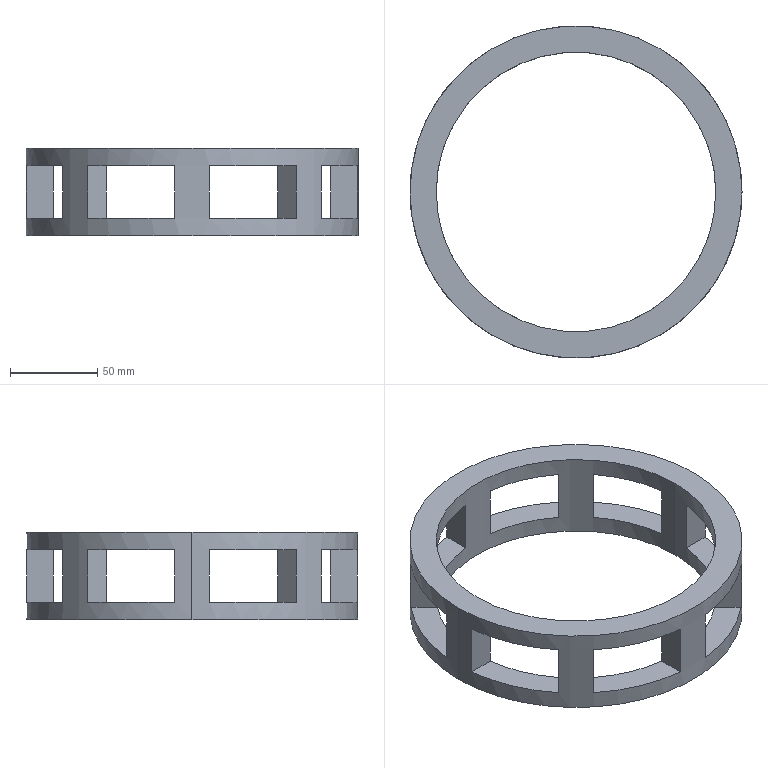Part | SolidWorks | features Cut 1, Extrusion 1 | 1 solid | 38 faces | box 190 x 190 x 50 mm | volume 237092 mm3 | plane 34 | cylinder 4 | commonest cylinder face diameters 160 x2 190 x2
STEP:
#1=CARTESIAN_POINT('',(-536.688,-139.054,40.));
#2=VERTEX_POINT('',#1);
#3=CARTESIAN_POINT('',(-520.512,-100.,40.));
#4=VERTEX_POINT('',#3);
#5=CARTESIAN_POINT('',(-599.884,-90.,40.));
#6=DIRECTION('',(0.,0.,1.));
#7=DIRECTION('',(1.,0.,0.));
#8=AXIS2_PLACEMENT_3D('',#5,#6,#7);
#9=CIRCLE('',#8,80.);
#10=EDGE_CURVE('',#2,#4,#9,.T.);
#11=ORIENTED_EDGE('',*,*,#10,.F.);
#12=CARTESIAN_POINT('',(-536.688,-139.054,10.));
#13=VERTEX_POINT('',#12);
#14=CARTESIAN_POINT('',(-536.688,-139.054,10.));
#15=DIRECTION('',(0.,0.,1.));
#16=VECTOR('',#15,1000.);
#17=LINE('',#14,#16);
#18=EDGE_CURVE('',#13,#2,#17,.T.);
#19=ORIENTED_EDGE('',*,*,#18,.F.);
#20=CARTESIAN_POINT('',(-520.512,-100.,10.));
#21=VERTEX_POINT('',#20);
#22=CARTESIAN_POINT('',(-599.884,-90.,10.));
#23=DIRECTION('',(0.,0.,1.));
#24=DIRECTION('',(1.,0.,0.));
#25=AXIS2_PLACEMENT_3D('',#22,#23,#24);
#26=CIRCLE('',#25,80.);
#27=EDGE_CURVE('',#13,#21,#26,.T.);
#28=ORIENTED_EDGE('',*,*,#27,.T.);
#29=CARTESIAN_POINT('',(-520.512,-100.,10.));
#30=DIRECTION('',(0.,0.,-1.));
#31=VECTOR('',#30,1000.);
#32=LINE('',#29,#31);
#33=EDGE_CURVE('',#4,#21,#32,.T.);
#34=ORIENTED_EDGE('',*,*,#33,.F.);
#35=EDGE_LOOP('',(#11,#19,#28,#34));
#36=FACE_BOUND('',#35,.T.);
#37=CARTESIAN_POINT('',(-589.884,-169.373,40.));
#38=VERTEX_POINT('',#37);
#39=CARTESIAN_POINT('',(-550.83,-153.196,40.));
#40=VERTEX_POINT('',#39);
#41=CARTESIAN_POINT('',(-599.884,-90.,40.));
#42=DIRECTION('',(0.,0.,1.));
#43=DIRECTION('',(1.,0.,0.));
#44=AXIS2_PLACEMENT_3D('',#41,#42,#43);
#45=CIRCLE('',#44,80.);
#46=EDGE_CURVE('',#38,#40,#45,.T.);
#47=ORIENTED_EDGE('',*,*,#46,.F.);
#48=CARTESIAN_POINT('',(-589.884,-169.373,10.));
#49=VERTEX_POINT('',#48);
#50=CARTESIAN_POINT('',(-589.884,-169.373,10.));
#51=DIRECTION('',(0.,0.,-1.));
#52=VECTOR('',#51,1000.);
#53=LINE('',#50,#52);
#54=EDGE_CURVE('',#38,#49,#53,.T.);
#55=ORIENTED_EDGE('',*,*,#54,.T.);
#56=CARTESIAN_POINT('',(-550.83,-153.196,10.));
#57=VERTEX_POINT('',#56);
#58=CARTESIAN_POINT('',(-599.884,-90.,10.));
#59=DIRECTION('',(0.,0.,1.));
#60=DIRECTION('',(1.,0.,0.));
#61=AXIS2_PLACEMENT_3D('',#58,#59,#60);
#62=CIRCLE('',#61,80.);
#63=EDGE_CURVE('',#49,#57,#62,.T.);
#64=ORIENTED_EDGE('',*,*,#63,.T.);
#65=CARTESIAN_POINT('',(-550.83,-153.196,10.));
#66=DIRECTION('',(0.,0.,1.));
#67=VECTOR('',#66,1000.);
#68=LINE('',#65,#67);
#69=EDGE_CURVE('',#57,#40,#68,.T.);
#70=ORIENTED_EDGE('',*,*,#69,.T.);
#71=EDGE_LOOP('',(#47,#55,#64,#70));
#72=FACE_BOUND('',#71,.T.);
#73=CARTESIAN_POINT('',(-648.938,-153.196,40.));
#74=VERTEX_POINT('',#73);
#75=CARTESIAN_POINT('',(-609.884,-169.373,40.));
#76=VERTEX_POINT('',#75);
#77=CARTESIAN_POINT('',(-599.884,-90.,40.));
#78=DIRECTION('',(0.,0.,1.));
#79=DIRECTION('',(1.,0.,0.));
#80=AXIS2_PLACEMENT_3D('',#77,#78,#79);
#81=CIRCLE('',#80,80.);
#82=EDGE_CURVE('',#74,#76,#81,.T.);
#83=ORIENTED_EDGE('',*,*,#82,.F.);
#84=CARTESIAN_POINT('',(-648.938,-153.196,10.));
#85=VERTEX_POINT('',#84);
#86=CARTESIAN_POINT('',(-648.938,-153.196,10.));
#87=DIRECTION('',(0.,0.,-1.));
#88=VECTOR('',#87,1000.);
#89=LINE('',#86,#88);
#90=EDGE_CURVE('',#74,#85,#89,.T.);
#91=ORIENTED_EDGE('',*,*,#90,.T.);
#92=CARTESIAN_POINT('',(-609.884,-169.373,10.));
#93=VERTEX_POINT('',#92);
#94=CARTESIAN_POINT('',(-599.884,-90.,10.));
#95=DIRECTION('',(0.,0.,1.));
#96=DIRECTION('',(1.,0.,0.));
#97=AXIS2_PLACEMENT_3D('',#94,#95,#96);
#98=CIRCLE('',#97,80.);
#99=EDGE_CURVE('',#85,#93,#98,.T.);
#100=ORIENTED_EDGE('',*,*,#99,.T.);
#101=CARTESIAN_POINT('',(-609.884,-169.373,10.));
#102=DIRECTION('',(0.,0.,-1.));
#103=VECTOR('',#102,1000.);
#104=LINE('',#101,#103);
#105=EDGE_CURVE('',#76,#93,#104,.T.);
#106=ORIENTED_EDGE('',*,*,#105,.F.);
#107=EDGE_LOOP('',(#83,#91,#100,#106));
#108=FACE_BOUND('',#107,.T.);
#109=CARTESIAN_POINT('',(-679.257,-100.,40.));
#110=VERTEX_POINT('',#109);
#111=CARTESIAN_POINT('',(-663.08,-139.054,40.));
#112=VERTEX_POINT('',#111);
#113=CARTESIAN_POINT('',(-599.884,-90.,40.));
#114=DIRECTION('',(0.,0.,1.));
#115=DIRECTION('',(1.,0.,0.));
#116=AXIS2_PLACEMENT_3D('',#113,#114,#115);
#117=CIRCLE('',#116,80.);
#118=EDGE_CURVE('',#110,#112,#117,.T.);
#119=ORIENTED_EDGE('',*,*,#118,.F.);
#120=CARTESIAN_POINT('',(-679.257,-100.,10.));
#121=VERTEX_POINT('',#120);
#122=CARTESIAN_POINT('',(-679.257,-100.,10.));
#123=DIRECTION('',(0.,0.,1.));
#124=VECTOR('',#123,1000.);
#125=LINE('',#122,#124);
#126=EDGE_CURVE('',#121,#110,#125,.T.);
#127=ORIENTED_EDGE('',*,*,#126,.F.);
#128=CARTESIAN_POINT('',(-663.08,-139.054,10.));
#129=VERTEX_POINT('',#128);
#130=CARTESIAN_POINT('',(-599.884,-90.,10.));
#131=DIRECTION('',(0.,0.,1.));
#132=DIRECTION('',(1.,0.,0.));
#133=AXIS2_PLACEMENT_3D('',#130,#131,#132);
#134=CIRCLE('',#133,80.);
#135=EDGE_CURVE('',#121,#129,#134,.T.);
#136=ORIENTED_EDGE('',*,*,#135,.T.);
#137=CARTESIAN_POINT('',(-663.08,-139.054,10.));
#138=DIRECTION('',(0.,0.,-1.));
#139=VECTOR('',#138,1000.);
#140=LINE('',#137,#139);
#141=EDGE_CURVE('',#112,#129,#140,.T.);
#142=ORIENTED_EDGE('',*,*,#141,.F.);
#143=EDGE_LOOP('',(#119,#127,#136,#142));
#144=FACE_BOUND('',#143,.T.);
#145=CARTESIAN_POINT('',(-679.884,-90.,50.));
#146=VERTEX_POINT('',#145);
#147=CARTESIAN_POINT('',(-519.884,-90.,50.));
#148=VERTEX_POINT('',#147);
#149=CARTESIAN_POINT('',(-599.884,-90.,50.));
#150=DIRECTION('',(0.,0.,1.));
#151=DIRECTION('',(1.,0.,0.));
#152=AXIS2_PLACEMENT_3D('',#149,#150,#151);
#153=CIRCLE('',#152,80.);
#154=EDGE_CURVE('',#146,#148,#153,.T.);
#155=ORIENTED_EDGE('',*,*,#154,.T.);
#156=CARTESIAN_POINT('',(-519.884,-90.,0.));
#157=VERTEX_POINT('',#156);
#158=CARTESIAN_POINT('',(-519.884,-90.,50.));
#159=DIRECTION('',(0.,0.,-1.));
#160=VECTOR('',#159,1000.);
#161=LINE('',#158,#160);
#162=EDGE_CURVE('',#148,#157,#161,.T.);
#163=ORIENTED_EDGE('',*,*,#162,.T.);
#164=CARTESIAN_POINT('',(-679.884,-90.,0.));
#165=VERTEX_POINT('',#164);
#166=CARTESIAN_POINT('',(-599.884,-90.,0.));
#167=DIRECTION('',(0.,0.,1.));
#168=DIRECTION('',(1.,0.,0.));
#169=AXIS2_PLACEMENT_3D('',#166,#167,#168);
#170=CIRCLE('',#169,80.);
#171=EDGE_CURVE('',#165,#157,#170,.T.);
#172=ORIENTED_EDGE('',*,*,#171,.F.);
#173=CARTESIAN_POINT('',(-679.884,-90.,50.));
#174=DIRECTION('',(0.,0.,-1.));
#175=VECTOR('',#174,1000.);
#176=LINE('',#173,#175);
#177=EDGE_CURVE('',#146,#165,#176,.T.);
#178=ORIENTED_EDGE('',*,*,#177,.F.);
#179=EDGE_LOOP('',(#155,#163,#172,#178));
#180=FACE_OUTER_BOUND('',#179,.T.);
#181=CARTESIAN_POINT('',(-599.884,-90.,50.));
#182=DIRECTION('',(0.,0.,-1.));
#183=DIRECTION('',(-1.,0.,0.));
#184=AXIS2_PLACEMENT_3D('',#181,#182,#183);
#185=CYLINDRICAL_SURFACE('',#184,80.);
#186=ADVANCED_FACE('',(#36,#72,#108,#144,#180),#185,.F.);
#187=CARTESIAN_POINT('',(-589.884,4.472,10.));
#188=VERTEX_POINT('',#187);
#189=CARTESIAN_POINT('',(-589.884,4.472,40.));
#190=VERTEX_POINT('',#189);
#191=CARTESIAN_POINT('',(-589.884,4.472,10.));
#192=DIRECTION('',(0.,0.,1.));
#193=VECTOR('',#192,1000.);
#194=LINE('',#191,#193);
#195=EDGE_CURVE('',#188,#190,#194,.T.);
#196=ORIENTED_EDGE('',*,*,#195,.F.);
#197=CARTESIAN_POINT('',(-540.153,-16.127,10.));
#198=VERTEX_POINT('',#197);
#199=CARTESIAN_POINT('',(-599.884,-90.,10.));
#200=DIRECTION('',(0.,0.,1.));
#201=DIRECTION('',(1.,0.,0.));
#202=AXIS2_PLACEMENT_3D('',#199,#200,#201);
#203=CIRCLE('',#202,95.);
#204=EDGE_CURVE('',#198,#188,#203,.T.);
#205=ORIENTED_EDGE('',*,*,#204,.F.);
#206=CARTESIAN_POINT('',(-540.153,-16.127,40.));
#207=VERTEX_POINT('',#206);
#208=CARTESIAN_POINT('',(-540.153,-16.127,10.));
#209=DIRECTION('',(0.,0.,1.));
#210=VECTOR('',#209,1000.);
#211=LINE('',#208,#210);
#212=EDGE_CURVE('',#198,#207,#211,.T.);
#213=ORIENTED_EDGE('',*,*,#212,.T.);
#214=CARTESIAN_POINT('',(-599.884,-90.,40.));
#215=DIRECTION('',(0.,0.,1.));
#216=DIRECTION('',(1.,0.,0.));
#217=AXIS2_PLACEMENT_3D('',#214,#215,#216);
#218=CIRCLE('',#217,95.);
#219=EDGE_CURVE('',#207,#190,#218,.T.);
#220=ORIENTED_EDGE('',*,*,#219,.T.);
#221=EDGE_LOOP('',(#196,#205,#213,#220));
#222=FACE_BOUND('',#221,.T.);
#223=CARTESIAN_POINT('',(-673.757,-30.269,10.));
#224=VERTEX_POINT('',#223);
#225=CARTESIAN_POINT('',(-673.757,-30.269,40.));
#226=VERTEX_POINT('',#225);
#227=CARTESIAN_POINT('',(-673.757,-30.269,10.));
#228=DIRECTION('',(0.,0.,1.));
#229=VECTOR('',#228,1000.);
#230=LINE('',#227,#229);
#231=EDGE_CURVE('',#224,#226,#230,.T.);
#232=ORIENTED_EDGE('',*,*,#231,.T.);
#233=CARTESIAN_POINT('',(-694.356,-80.,40.));
#234=VERTEX_POINT('',#233);
#235=CARTESIAN_POINT('',(-599.884,-90.,40.));
#236=DIRECTION('',(0.,0.,1.));
#237=DIRECTION('',(1.,0.,0.));
#238=AXIS2_PLACEMENT_3D('',#235,#236,#237);
#239=CIRCLE('',#238,95.);
#240=EDGE_CURVE('',#226,#234,#239,.T.);
#241=ORIENTED_EDGE('',*,*,#240,.T.);
#242=CARTESIAN_POINT('',(-694.356,-80.,10.));
#243=VERTEX_POINT('',#242);
#244=CARTESIAN_POINT('',(-694.356,-80.,10.));
#245=DIRECTION('',(0.,0.,1.));
#246=VECTOR('',#245,1000.);
#247=LINE('',#244,#246);
#248=EDGE_CURVE('',#243,#234,#247,.T.);
#249=ORIENTED_EDGE('',*,*,#248,.F.);
#250=CARTESIAN_POINT('',(-599.884,-90.,10.));
#251=DIRECTION('',(0.,0.,1.));
#252=DIRECTION('',(1.,0.,0.));
#253=AXIS2_PLACEMENT_3D('',#250,#251,#252);
#254=CIRCLE('',#253,95.);
#255=EDGE_CURVE('',#224,#243,#254,.T.);
#256=ORIENTED_EDGE('',*,*,#255,.F.);
#257=EDGE_LOOP('',(#232,#241,#249,#256));
#258=FACE_BOUND('',#257,.T.);
#259=CARTESIAN_POINT('',(-526.011,-30.269,10.));
#260=VERTEX_POINT('',#259);
#261=CARTESIAN_POINT('',(-526.011,-30.269,40.));
#262=VERTEX_POINT('',#261);
#263=CARTESIAN_POINT('',(-526.011,-30.269,10.));
#264=DIRECTION('',(0.,0.,1.));
#265=VECTOR('',#264,1000.);
#266=LINE('',#263,#265);
#267=EDGE_CURVE('',#260,#262,#266,.T.);
#268=ORIENTED_EDGE('',*,*,#267,.F.);
#269=CARTESIAN_POINT('',(-505.412,-80.,10.));
#270=VERTEX_POINT('',#269);
#271=CARTESIAN_POINT('',(-599.884,-90.,10.));
#272=DIRECTION('',(0.,0.,1.));
#273=DIRECTION('',(1.,0.,0.));
#274=AXIS2_PLACEMENT_3D('',#271,#272,#273);
#275=CIRCLE('',#274,95.);
#276=EDGE_CURVE('',#270,#260,#275,.T.);
#277=ORIENTED_EDGE('',*,*,#276,.F.);
#278=CARTESIAN_POINT('',(-505.412,-80.,40.));
#279=VERTEX_POINT('',#278);
#280=CARTESIAN_POINT('',(-505.412,-80.,10.));
#281=DIRECTION('',(0.,0.,1.));
#282=VECTOR('',#281,1000.);
#283=LINE('',#280,#282);
#284=EDGE_CURVE('',#270,#279,#283,.T.);
#285=ORIENTED_EDGE('',*,*,#284,.T.);
#286=CARTESIAN_POINT('',(-599.884,-90.,40.));
#287=DIRECTION('',(0.,0.,1.));
#288=DIRECTION('',(1.,0.,0.));
#289=AXIS2_PLACEMENT_3D('',#286,#287,#288);
#290=CIRCLE('',#289,95.);
#291=EDGE_CURVE('',#279,#262,#290,.T.);
#292=ORIENTED_EDGE('',*,*,#291,.T.);
#293=EDGE_LOOP('',(#268,#277,#285,#292));
#294=FACE_BOUND('',#293,.T.);
#295=CARTESIAN_POINT('',(-609.884,4.472,40.));
#296=VERTEX_POINT('',#295);
#297=CARTESIAN_POINT('',(-659.615,-16.127,40.));
#298=VERTEX_POINT('',#297);
#299=CARTESIAN_POINT('',(-599.884,-90.,40.));
#300=DIRECTION('',(0.,0.,1.));
#301=DIRECTION('',(1.,0.,0.));
#302=AXIS2_PLACEMENT_3D('',#299,#300,#301);
#303=CIRCLE('',#302,95.);
#304=EDGE_CURVE('',#296,#298,#303,.T.);
#305=ORIENTED_EDGE('',*,*,#304,.T.);
#306=CARTESIAN_POINT('',(-659.615,-16.127,10.));
#307=VERTEX_POINT('',#306);
#308=CARTESIAN_POINT('',(-659.615,-16.127,10.));
#309=DIRECTION('',(0.,0.,1.));
#310=VECTOR('',#309,1000.);
#311=LINE('',#308,#310);
#312=EDGE_CURVE('',#307,#298,#311,.T.);
#313=ORIENTED_EDGE('',*,*,#312,.F.);
#314=CARTESIAN_POINT('',(-609.884,4.472,10.));
#315=VERTEX_POINT('',#314);
#316=CARTESIAN_POINT('',(-599.884,-90.,10.));
#317=DIRECTION('',(0.,0.,1.));
#318=DIRECTION('',(1.,0.,0.));
#319=AXIS2_PLACEMENT_3D('',#316,#317,#318);
#320=CIRCLE('',#319,95.);
#321=EDGE_CURVE('',#315,#307,#320,.T.);
#322=ORIENTED_EDGE('',*,*,#321,.F.);
#323=CARTESIAN_POINT('',(-609.884,4.472,10.));
#324=DIRECTION('',(0.,0.,1.));
#325=VECTOR('',#324,1000.);
#326=LINE('',#323,#325);
#327=EDGE_CURVE('',#315,#296,#326,.T.);
#328=ORIENTED_EDGE('',*,*,#327,.T.);
#329=EDGE_LOOP('',(#305,#313,#322,#328));
#330=FACE_BOUND('',#329,.T.);
#331=CARTESIAN_POINT('',(-504.884,-90.,50.));
#332=VERTEX_POINT('',#331);
#333=CARTESIAN_POINT('',(-694.884,-90.,50.));
#334=VERTEX_POINT('',#333);
#335=CARTESIAN_POINT('',(-599.884,-90.,50.));
#336=DIRECTION('',(0.,0.,1.));
#337=DIRECTION('',(1.,0.,0.));
#338=AXIS2_PLACEMENT_3D('',#335,#336,#337);
#339=CIRCLE('',#338,95.);
#340=EDGE_CURVE('',#332,#334,#339,.T.);
#341=ORIENTED_EDGE('',*,*,#340,.F.);
#342=CARTESIAN_POINT('',(-504.884,-90.,0.));
#343=VERTEX_POINT('',#342);
#344=CARTESIAN_POINT('',(-504.884,-90.,50.));
#345=DIRECTION('',(0.,0.,-1.));
#346=VECTOR('',#345,1000.);
#347=LINE('',#344,#346);
#348=EDGE_CURVE('',#332,#343,#347,.T.);
#349=ORIENTED_EDGE('',*,*,#348,.T.);
#350=CARTESIAN_POINT('',(-694.884,-90.,0.));
#351=VERTEX_POINT('',#350);
#352=CARTESIAN_POINT('',(-599.884,-90.,0.));
#353=DIRECTION('',(0.,0.,1.));
#354=DIRECTION('',(1.,0.,0.));
#355=AXIS2_PLACEMENT_3D('',#352,#353,#354);
#356=CIRCLE('',#355,95.);
#357=EDGE_CURVE('',#343,#351,#356,.T.);
#358=ORIENTED_EDGE('',*,*,#357,.T.);
#359=CARTESIAN_POINT('',(-694.884,-90.,50.));
#360=DIRECTION('',(0.,0.,-1.));
#361=VECTOR('',#360,1000.);
#362=LINE('',#359,#361);
#363=EDGE_CURVE('',#334,#351,#362,.T.);
#364=ORIENTED_EDGE('',*,*,#363,.F.);
#365=EDGE_LOOP('',(#341,#349,#358,#364));
#366=FACE_OUTER_BOUND('',#365,.T.);
#367=CARTESIAN_POINT('',(-599.884,-90.,50.));
#368=DIRECTION('',(0.,0.,-1.));
#369=DIRECTION('',(-1.,0.,0.));
#370=AXIS2_PLACEMENT_3D('',#367,#368,#369);
#371=CYLINDRICAL_SURFACE('',#370,95.);
#372=ADVANCED_FACE('',(#222,#258,#294,#330,#366),#371,.T.);
#373=ORIENTED_EDGE('',*,*,#348,.F.);
#374=CARTESIAN_POINT('',(-599.884,-90.,50.));
#375=DIRECTION('',(0.,0.,1.));
#376=DIRECTION('',(1.,0.,0.));
#377=AXIS2_PLACEMENT_3D('',#374,#375,#376);
#378=CIRCLE('',#377,95.);
#379=EDGE_CURVE('',#334,#332,#378,.T.);
#380=ORIENTED_EDGE('',*,*,#379,.F.);
#381=ORIENTED_EDGE('',*,*,#363,.T.);
#382=CARTESIAN_POINT('',(-599.884,-90.,0.));
#383=DIRECTION('',(0.,0.,1.));
#384=DIRECTION('',(1.,0.,0.));
#385=AXIS2_PLACEMENT_3D('',#382,#383,#384);
#386=CIRCLE('',#385,95.);
#387=EDGE_CURVE('',#351,#343,#386,.T.);
#388=ORIENTED_EDGE('',*,*,#387,.T.);
#389=EDGE_LOOP('',(#373,#380,#381,#388));
#390=FACE_OUTER_BOUND('',#389,.T.);
#391=CARTESIAN_POINT('',(-694.356,-100.,10.));
#392=VERTEX_POINT('',#391);
#393=CARTESIAN_POINT('',(-694.356,-100.,40.));
#394=VERTEX_POINT('',#393);
#395=CARTESIAN_POINT('',(-694.356,-100.,10.));
#396=DIRECTION('',(0.,0.,1.));
#397=VECTOR('',#396,1000.);
#398=LINE('',#395,#397);
#399=EDGE_CURVE('',#392,#394,#398,.T.);
#400=ORIENTED_EDGE('',*,*,#399,.T.);
#401=CARTESIAN_POINT('',(-673.757,-149.731,40.));
#402=VERTEX_POINT('',#401);
#403=CARTESIAN_POINT('',(-599.884,-90.,40.));
#404=DIRECTION('',(0.,0.,1.));
#405=DIRECTION('',(1.,0.,0.));
#406=AXIS2_PLACEMENT_3D('',#403,#404,#405);
#407=CIRCLE('',#406,95.);
#408=EDGE_CURVE('',#394,#402,#407,.T.);
#409=ORIENTED_EDGE('',*,*,#408,.T.);
#410=CARTESIAN_POINT('',(-673.757,-149.731,10.));
#411=VERTEX_POINT('',#410);
#412=CARTESIAN_POINT('',(-673.757,-149.731,10.));
#413=DIRECTION('',(0.,0.,1.));
#414=VECTOR('',#413,1000.);
#415=LINE('',#412,#414);
#416=EDGE_CURVE('',#411,#402,#415,.T.);
#417=ORIENTED_EDGE('',*,*,#416,.F.);
#418=CARTESIAN_POINT('',(-599.884,-90.,10.));
#419=DIRECTION('',(0.,0.,1.));
#420=DIRECTION('',(1.,0.,0.));
#421=AXIS2_PLACEMENT_3D('',#418,#419,#420);
#422=CIRCLE('',#421,95.);
#423=EDGE_CURVE('',#392,#411,#422,.T.);
#424=ORIENTED_EDGE('',*,*,#423,.F.);
#425=EDGE_LOOP('',(#400,#409,#417,#424));
#426=FACE_BOUND('',#425,.T.);
#427=CARTESIAN_POINT('',(-526.011,-149.731,40.));
#428=VERTEX_POINT('',#427);
#429=CARTESIAN_POINT('',(-505.412,-100.,40.));
#430=VERTEX_POINT('',#429);
#431=CARTESIAN_POINT('',(-599.884,-90.,40.));
#432=DIRECTION('',(0.,0.,1.));
#433=DIRECTION('',(1.,0.,0.));
#434=AXIS2_PLACEMENT_3D('',#431,#432,#433);
#435=CIRCLE('',#434,95.);
#436=EDGE_CURVE('',#428,#430,#435,.T.);
#437=ORIENTED_EDGE('',*,*,#436,.T.);
#438=CARTESIAN_POINT('',(-505.412,-100.,10.));
#439=VERTEX_POINT('',#438);
#440=CARTESIAN_POINT('',(-505.412,-100.,10.));
#441=DIRECTION('',(0.,0.,1.));
#442=VECTOR('',#441,1000.);
#443=LINE('',#440,#442);
#444=EDGE_CURVE('',#439,#430,#443,.T.);
#445=ORIENTED_EDGE('',*,*,#444,.F.);
#446=CARTESIAN_POINT('',(-526.011,-149.731,10.));
#447=VERTEX_POINT('',#446);
#448=CARTESIAN_POINT('',(-599.884,-90.,10.));
#449=DIRECTION('',(0.,0.,1.));
#450=DIRECTION('',(1.,0.,0.));
#451=AXIS2_PLACEMENT_3D('',#448,#449,#450);
#452=CIRCLE('',#451,95.);
#453=EDGE_CURVE('',#447,#439,#452,.T.);
#454=ORIENTED_EDGE('',*,*,#453,.F.);
#455=CARTESIAN_POINT('',(-526.011,-149.731,10.));
#456=DIRECTION('',(0.,0.,1.));
#457=VECTOR('',#456,1000.);
#458=LINE('',#455,#457);
#459=EDGE_CURVE('',#447,#428,#458,.T.);
#460=ORIENTED_EDGE('',*,*,#459,.T.);
#461=EDGE_LOOP('',(#437,#445,#454,#460));
#462=FACE_BOUND('',#461,.T.);
#463=CARTESIAN_POINT('',(-659.615,-163.873,40.));
#464=VERTEX_POINT('',#463);
#465=CARTESIAN_POINT('',(-609.884,-184.472,40.));
#466=VERTEX_POINT('',#465);
#467=CARTESIAN_POINT('',(-599.884,-90.,40.));
#468=DIRECTION('',(0.,0.,1.));
#469=DIRECTION('',(1.,0.,0.));
#470=AXIS2_PLACEMENT_3D('',#467,#468,#469);
#471=CIRCLE('',#470,95.);
#472=EDGE_CURVE('',#464,#466,#471,.T.);
#473=ORIENTED_EDGE('',*,*,#472,.T.);
#474=CARTESIAN_POINT('',(-609.884,-184.472,10.));
#475=VERTEX_POINT('',#474);
#476=CARTESIAN_POINT('',(-609.884,-184.472,10.));
#477=DIRECTION('',(0.,0.,1.));
#478=VECTOR('',#477,1000.);
#479=LINE('',#476,#478);
#480=EDGE_CURVE('',#475,#466,#479,.T.);
#481=ORIENTED_EDGE('',*,*,#480,.F.);
#482=CARTESIAN_POINT('',(-659.615,-163.873,10.));
#483=VERTEX_POINT('',#482);
#484=CARTESIAN_POINT('',(-599.884,-90.,10.));
#485=DIRECTION('',(0.,0.,1.));
#486=DIRECTION('',(1.,0.,0.));
#487=AXIS2_PLACEMENT_3D('',#484,#485,#486);
#488=CIRCLE('',#487,95.);
#489=EDGE_CURVE('',#483,#475,#488,.T.);
#490=ORIENTED_EDGE('',*,*,#489,.F.);
#491=CARTESIAN_POINT('',(-659.615,-163.873,10.));
#492=DIRECTION('',(0.,0.,1.));
#493=VECTOR('',#492,1000.);
#494=LINE('',#491,#493);
#495=EDGE_CURVE('',#483,#464,#494,.T.);
#496=ORIENTED_EDGE('',*,*,#495,.T.);
#497=EDGE_LOOP('',(#473,#481,#490,#496));
#498=FACE_BOUND('',#497,.T.);
#499=CARTESIAN_POINT('',(-540.153,-163.873,10.));
#500=VERTEX_POINT('',#499);
#501=CARTESIAN_POINT('',(-540.153,-163.873,40.));
#502=VERTEX_POINT('',#501);
#503=CARTESIAN_POINT('',(-540.153,-163.873,10.));
#504=DIRECTION('',(0.,0.,1.));
#505=VECTOR('',#504,1000.);
#506=LINE('',#503,#505);
#507=EDGE_CURVE('',#500,#502,#506,.T.);
#508=ORIENTED_EDGE('',*,*,#507,.F.);
#509=CARTESIAN_POINT('',(-589.884,-184.472,10.));
#510=VERTEX_POINT('',#509);
#511=CARTESIAN_POINT('',(-599.884,-90.,10.));
#512=DIRECTION('',(0.,0.,1.));
#513=DIRECTION('',(1.,0.,0.));
#514=AXIS2_PLACEMENT_3D('',#511,#512,#513);
#515=CIRCLE('',#514,95.);
#516=EDGE_CURVE('',#510,#500,#515,.T.);
#517=ORIENTED_EDGE('',*,*,#516,.F.);
#518=CARTESIAN_POINT('',(-589.884,-184.472,40.));
#519=VERTEX_POINT('',#518);
#520=CARTESIAN_POINT('',(-589.884,-184.472,10.));
#521=DIRECTION('',(0.,0.,1.));
#522=VECTOR('',#521,1000.);
#523=LINE('',#520,#522);
#524=EDGE_CURVE('',#510,#519,#523,.T.);
#525=ORIENTED_EDGE('',*,*,#524,.T.);
#526=CARTESIAN_POINT('',(-599.884,-90.,40.));
#527=DIRECTION('',(0.,0.,1.));
#528=DIRECTION('',(1.,0.,0.));
#529=AXIS2_PLACEMENT_3D('',#526,#527,#528);
#530=CIRCLE('',#529,95.);
#531=EDGE_CURVE('',#519,#502,#530,.T.);
#532=ORIENTED_EDGE('',*,*,#531,.T.);
#533=EDGE_LOOP('',(#508,#517,#525,#532));
#534=FACE_BOUND('',#533,.T.);
#535=CARTESIAN_POINT('',(-599.884,-90.,50.));
#536=DIRECTION('',(0.,0.,-1.));
#537=DIRECTION('',(-1.,0.,0.));
#538=AXIS2_PLACEMENT_3D('',#535,#536,#537);
#539=CYLINDRICAL_SURFACE('',#538,95.);
#540=ADVANCED_FACE('',(#390,#426,#462,#498,#534),#539,.T.);
#541=ORIENTED_EDGE('',*,*,#162,.F.);
#542=CARTESIAN_POINT('',(-599.884,-90.,50.));
#543=DIRECTION('',(0.,0.,1.));
#544=DIRECTION('',(1.,0.,0.));
#545=AXIS2_PLACEMENT_3D('',#542,#543,#544);
#546=CIRCLE('',#545,80.);
#547=EDGE_CURVE('',#148,#146,#546,.T.);
#548=ORIENTED_EDGE('',*,*,#547,.T.);
#549=ORIENTED_EDGE('',*,*,#177,.T.);
#550=CARTESIAN_POINT('',(-599.884,-90.,0.));
#551=DIRECTION('',(0.,0.,1.));
#552=DIRECTION('',(1.,0.,0.));
#553=AXIS2_PLACEMENT_3D('',#550,#551,#552);
#554=CIRCLE('',#553,80.);
#555=EDGE_CURVE('',#157,#165,#554,.T.);
#556=ORIENTED_EDGE('',*,*,#555,.F.);
#557=EDGE_LOOP('',(#541,#548,#549,#556));
#558=FACE_OUTER_BOUND('',#557,.T.);
#559=CARTESIAN_POINT('',(-550.83,-26.804,40.));
#560=VERTEX_POINT('',#559);
#561=CARTESIAN_POINT('',(-589.884,-10.627,40.));
#562=VERTEX_POINT('',#561);
#563=CARTESIAN_POINT('',(-599.884,-90.,40.));
#564=DIRECTION('',(0.,0.,1.));
#565=DIRECTION('',(1.,0.,0.));
#566=AXIS2_PLACEMENT_3D('',#563,#564,#565);
#567=CIRCLE('',#566,80.);
#568=EDGE_CURVE('',#560,#562,#567,.T.);
#569=ORIENTED_EDGE('',*,*,#568,.F.);
#570=CARTESIAN_POINT('',(-550.83,-26.804,10.));
#571=VERTEX_POINT('',#570);
#572=CARTESIAN_POINT('',(-550.83,-26.804,10.));
#573=DIRECTION('',(0.,0.,1.));
#574=VECTOR('',#573,1000.);
#575=LINE('',#572,#574);
#576=EDGE_CURVE('',#571,#560,#575,.T.);
#577=ORIENTED_EDGE('',*,*,#576,.F.);
#578=CARTESIAN_POINT('',(-589.884,-10.627,10.));
#579=VERTEX_POINT('',#578);
#580=CARTESIAN_POINT('',(-599.884,-90.,10.));
#581=DIRECTION('',(0.,0.,1.));
#582=DIRECTION('',(1.,0.,0.));
#583=AXIS2_PLACEMENT_3D('',#580,#581,#582);
#584=CIRCLE('',#583,80.);
#585=EDGE_CURVE('',#571,#579,#584,.T.);
#586=ORIENTED_EDGE('',*,*,#585,.T.);
#587=CARTESIAN_POINT('',(-589.884,-10.627,10.));
#588=DIRECTION('',(0.,0.,1.));
#589=VECTOR('',#588,1000.);
#590=LINE('',#587,#589);
#591=EDGE_CURVE('',#579,#562,#590,.T.);
#592=ORIENTED_EDGE('',*,*,#591,.T.);
#593=EDGE_LOOP('',(#569,#577,#586,#592));
#594=FACE_BOUND('',#593,.T.);
#595=CARTESIAN_POINT('',(-609.884,-10.627,40.));
#596=VERTEX_POINT('',#595);
#597=CARTESIAN_POINT('',(-648.938,-26.804,40.));
#598=VERTEX_POINT('',#597);
#599=CARTESIAN_POINT('',(-599.884,-90.,40.));
#600=DIRECTION('',(0.,0.,1.));
#601=DIRECTION('',(1.,0.,0.));
#602=AXIS2_PLACEMENT_3D('',#599,#600,#601);
#603=CIRCLE('',#602,80.);
#604=EDGE_CURVE('',#596,#598,#603,.T.);
#605=ORIENTED_EDGE('',*,*,#604,.F.);
#606=CARTESIAN_POINT('',(-609.884,-10.627,10.));
#607=VERTEX_POINT('',#606);
#608=CARTESIAN_POINT('',(-609.884,-10.627,10.));
#609=DIRECTION('',(0.,0.,1.));
#610=VECTOR('',#609,1000.);
#611=LINE('',#608,#610);
#612=EDGE_CURVE('',#607,#596,#611,.T.);
#613=ORIENTED_EDGE('',*,*,#612,.F.);
#614=CARTESIAN_POINT('',(-648.938,-26.804,10.));
#615=VERTEX_POINT('',#614);
#616=CARTESIAN_POINT('',(-599.884,-90.,10.));
#617=DIRECTION('',(0.,0.,1.));
#618=DIRECTION('',(1.,0.,0.));
#619=AXIS2_PLACEMENT_3D('',#616,#617,#618);
#620=CIRCLE('',#619,80.);
#621=EDGE_CURVE('',#607,#615,#620,.T.);
#622=ORIENTED_EDGE('',*,*,#621,.T.);
#623=CARTESIAN_POINT('',(-648.938,-26.804,10.));
#624=DIRECTION('',(0.,0.,-1.));
#625=VECTOR('',#624,1000.);
#626=LINE('',#623,#625);
#627=EDGE_CURVE('',#598,#615,#626,.T.);
#628=ORIENTED_EDGE('',*,*,#627,.F.);
#629=EDGE_LOOP('',(#605,#613,#622,#628));
#630=FACE_BOUND('',#629,.T.);
#631=CARTESIAN_POINT('',(-663.08,-40.946,40.));
#632=VERTEX_POINT('',#631);
#633=CARTESIAN_POINT('',(-679.257,-80.,40.));
#634=VERTEX_POINT('',#633);
#635=CARTESIAN_POINT('',(-599.884,-90.,40.));
#636=DIRECTION('',(0.,0.,1.));
#637=DIRECTION('',(1.,0.,0.));
#638=AXIS2_PLACEMENT_3D('',#635,#636,#637);
#639=CIRCLE('',#638,80.);
#640=EDGE_CURVE('',#632,#634,#639,.T.);
#641=ORIENTED_EDGE('',*,*,#640,.F.);
#642=CARTESIAN_POINT('',(-663.08,-40.946,10.));
#643=VERTEX_POINT('',#642);
#644=CARTESIAN_POINT('',(-663.08,-40.946,10.));
#645=DIRECTION('',(0.,0.,-1.));
#646=VECTOR('',#645,1000.);
#647=LINE('',#644,#646);
#648=EDGE_CURVE('',#632,#643,#647,.T.);
#649=ORIENTED_EDGE('',*,*,#648,.T.);
#650=CARTESIAN_POINT('',(-679.257,-80.,10.));
#651=VERTEX_POINT('',#650);
#652=CARTESIAN_POINT('',(-599.884,-90.,10.));
#653=DIRECTION('',(0.,0.,1.));
#654=DIRECTION('',(1.,0.,0.));
#655=AXIS2_PLACEMENT_3D('',#652,#653,#654);
#656=CIRCLE('',#655,80.);
#657=EDGE_CURVE('',#643,#651,#656,.T.);
#658=ORIENTED_EDGE('',*,*,#657,.T.);
#659=CARTESIAN_POINT('',(-679.257,-80.,10.));
#660=DIRECTION('',(0.,0.,1.));
#661=VECTOR('',#660,1000.);
#662=LINE('',#659,#661);
#663=EDGE_CURVE('',#651,#634,#662,.T.);
#664=ORIENTED_EDGE('',*,*,#663,.T.);
#665=EDGE_LOOP('',(#641,#649,#658,#664));
#666=FACE_BOUND('',#665,.T.);
#667=CARTESIAN_POINT('',(-536.688,-40.946,10.));
#668=VERTEX_POINT('',#667);
#669=CARTESIAN_POINT('',(-536.688,-40.946,40.));
#670=VERTEX_POINT('',#669);
#671=CARTESIAN_POINT('',(-536.688,-40.946,10.));
#672=DIRECTION('',(0.,0.,1.));
#673=VECTOR('',#672,1000.);
#674=LINE('',#671,#673);
#675=EDGE_CURVE('',#668,#670,#674,.T.);
#676=ORIENTED_EDGE('',*,*,#675,.T.);
#677=CARTESIAN_POINT('',(-520.512,-80.,40.));
#678=VERTEX_POINT('',#677);
#679=CARTESIAN_POINT('',(-599.884,-90.,40.));
#680=DIRECTION('',(0.,0.,1.));
#681=DIRECTION('',(1.,0.,0.));
#682=AXIS2_PLACEMENT_3D('',#679,#680,#681);
#683=CIRCLE('',#682,80.);
#684=EDGE_CURVE('',#678,#670,#683,.T.);
#685=ORIENTED_EDGE('',*,*,#684,.F.);
#686=CARTESIAN_POINT('',(-520.512,-80.,10.));
#687=VERTEX_POINT('',#686);
#688=CARTESIAN_POINT('',(-520.512,-80.,10.));
#689=DIRECTION('',(0.,0.,-1.));
#690=VECTOR('',#689,1000.);
#691=LINE('',#688,#690);
#692=EDGE_CURVE('',#678,#687,#691,.T.);
#693=ORIENTED_EDGE('',*,*,#692,.T.);
#694=CARTESIAN_POINT('',(-599.884,-90.,10.));
#695=DIRECTION('',(0.,0.,1.));
#696=DIRECTION('',(1.,0.,0.));
#697=AXIS2_PLACEMENT_3D('',#694,#695,#696);
#698=CIRCLE('',#697,80.);
#699=EDGE_CURVE('',#687,#668,#698,.T.);
#700=ORIENTED_EDGE('',*,*,#699,.T.);
#701=EDGE_LOOP('',(#676,#685,#693,#700));
#702=FACE_BOUND('',#701,.T.);
#703=CARTESIAN_POINT('',(-599.884,-90.,50.));
#704=DIRECTION('',(0.,0.,-1.));
#705=DIRECTION('',(-1.,0.,0.));
#706=AXIS2_PLACEMENT_3D('',#703,#704,#705);
#707=CYLINDRICAL_SURFACE('',#706,80.);
#708=ADVANCED_FACE('',(#558,#594,#630,#666,#702),#707,.F.);
#709=ORIENTED_EDGE('',*,*,#379,.T.);
#710=ORIENTED_EDGE('',*,*,#340,.T.);
#711=EDGE_LOOP('',(#709,#710));
#712=FACE_OUTER_BOUND('',#711,.T.);
#713=ORIENTED_EDGE('',*,*,#154,.F.);
#714=ORIENTED_EDGE('',*,*,#547,.F.);
#715=EDGE_LOOP('',(#713,#714));
#716=FACE_BOUND('',#715,.T.);
#717=CARTESIAN_POINT('',(-599.884,-90.,50.));
#718=DIRECTION('',(0.,0.,1.));
#719=DIRECTION('',(1.,0.,0.));
#720=AXIS2_PLACEMENT_3D('',#717,#718,#719);
#721=PLANE('',#720);
#722=ADVANCED_FACE('',(#712,#716),#721,.T.);
#723=ORIENTED_EDGE('',*,*,#387,.F.);
#724=ORIENTED_EDGE('',*,*,#357,.F.);
#725=EDGE_LOOP('',(#723,#724));
#726=FACE_OUTER_BOUND('',#725,.T.);
#727=ORIENTED_EDGE('',*,*,#171,.T.);
#728=ORIENTED_EDGE('',*,*,#555,.T.);
#729=EDGE_LOOP('',(#727,#728));
#730=FACE_BOUND('',#729,.T.);
#731=CARTESIAN_POINT('',(-599.884,-90.,0.));
#732=DIRECTION('',(0.,0.,1.));
#733=DIRECTION('',(1.,0.,0.));
#734=AXIS2_PLACEMENT_3D('',#731,#732,#733);
#735=PLANE('',#734);
#736=ADVANCED_FACE('',(#726,#730),#735,.F.);
#737=ORIENTED_EDGE('',*,*,#105,.T.);
#738=CARTESIAN_POINT('',(-609.884,0.,10.));
#739=DIRECTION('',(0.,1.,0.));
#740=VECTOR('',#739,1000.);
#741=LINE('',#738,#740);
#742=EDGE_CURVE('',#475,#93,#741,.T.);
#743=ORIENTED_EDGE('',*,*,#742,.F.);
#744=ORIENTED_EDGE('',*,*,#480,.T.);
#745=CARTESIAN_POINT('',(-609.884,0.,40.));
#746=DIRECTION('',(0.,1.,0.));
#747=VECTOR('',#746,1000.);
#748=LINE('',#745,#747);
#749=EDGE_CURVE('',#466,#76,#748,.T.);
#750=ORIENTED_EDGE('',*,*,#749,.T.);
#751=EDGE_LOOP('',(#737,#743,#744,#750));
#752=FACE_OUTER_BOUND('',#751,.T.);
#753=CARTESIAN_POINT('',(-609.884,0.,10.));
#754=DIRECTION('',(1.,0.,0.));
#755=DIRECTION('',(0.,0.,-1.));
#756=AXIS2_PLACEMENT_3D('',#753,#754,#755);
#757=PLANE('',#756);
#758=ADVANCED_FACE('',(#752),#757,.F.);
#759=CARTESIAN_POINT('',(-247.871,247.871,40.));
#760=DIRECTION('',(0.7071,0.7071,0.));
#761=VECTOR('',#760,1000.);
#762=LINE('',#759,#761);
#763=EDGE_CURVE('',#464,#74,#762,.T.);
#764=ORIENTED_EDGE('',*,*,#763,.F.);
#765=ORIENTED_EDGE('',*,*,#495,.F.);
#766=CARTESIAN_POINT('',(-247.871,247.871,10.));
#767=DIRECTION('',(0.7071,0.7071,0.));
#768=VECTOR('',#767,1000.);
#769=LINE('',#766,#768);
#770=EDGE_CURVE('',#483,#85,#769,.T.);
#771=ORIENTED_EDGE('',*,*,#770,.T.);
#772=ORIENTED_EDGE('',*,*,#90,.F.);
#773=EDGE_LOOP('',(#764,#765,#771,#772));
#774=FACE_OUTER_BOUND('',#773,.T.);
#775=CARTESIAN_POINT('',(-247.871,247.871,10.));
#776=DIRECTION('',(0.7071,-0.7071,0.));
#777=DIRECTION('',(0.7071,0.7071,0.));
#778=AXIS2_PLACEMENT_3D('',#775,#776,#777);
#779=PLANE('',#778);
#780=ADVANCED_FACE('',(#774),#779,.T.);
#781=ORIENTED_EDGE('',*,*,#770,.F.);
#782=ORIENTED_EDGE('',*,*,#489,.T.);
#783=ORIENTED_EDGE('',*,*,#742,.T.);
#784=ORIENTED_EDGE('',*,*,#99,.F.);
#785=EDGE_LOOP('',(#781,#782,#783,#784));
#786=FACE_OUTER_BOUND('',#785,.T.);
#787=CARTESIAN_POINT('',(0.,0.,10.));
#788=DIRECTION('',(0.,0.,1.));
#789=DIRECTION('',(1.,0.,0.));
#790=AXIS2_PLACEMENT_3D('',#787,#788,#789);
#791=PLANE('',#790);
#792=ADVANCED_FACE('',(#786),#791,.T.);
#793=ORIENTED_EDGE('',*,*,#82,.T.);
#794=ORIENTED_EDGE('',*,*,#749,.F.);
#795=ORIENTED_EDGE('',*,*,#472,.F.);
#796=ORIENTED_EDGE('',*,*,#763,.T.);
#797=EDGE_LOOP('',(#793,#794,#795,#796));
#798=FACE_OUTER_BOUND('',#797,.T.);
#799=CARTESIAN_POINT('',(0.,0.,40.));
#800=DIRECTION('',(0.,0.,1.));
#801=DIRECTION('',(1.,0.,0.));
#802=AXIS2_PLACEMENT_3D('',#799,#800,#801);
#803=PLANE('',#802);
#804=ADVANCED_FACE('',(#798),#803,.F.);
#805=CARTESIAN_POINT('',(0.,-80.,10.));
#806=DIRECTION('',(-1.,0.,0.));
#807=VECTOR('',#806,1000.);
#808=LINE('',#805,#807);
#809=EDGE_CURVE('',#651,#243,#808,.T.);
#810=ORIENTED_EDGE('',*,*,#809,.T.);
#811=ORIENTED_EDGE('',*,*,#248,.T.);
#812=CARTESIAN_POINT('',(0.,-80.,40.));
#813=DIRECTION('',(-1.,0.,0.));
#814=VECTOR('',#813,1000.);
#815=LINE('',#812,#814);
#816=EDGE_CURVE('',#634,#234,#815,.T.);
#817=ORIENTED_EDGE('',*,*,#816,.F.);
#818=ORIENTED_EDGE('',*,*,#663,.F.);
#819=EDGE_LOOP('',(#810,#811,#817,#818));
#820=FACE_OUTER_BOUND('',#819,.T.);
#821=CARTESIAN_POINT('',(0.,-80.,10.));
#822=DIRECTION('',(0.,1.,0.));
#823=DIRECTION('',(0.,0.,1.));
#824=AXIS2_PLACEMENT_3D('',#821,#822,#823);
#825=PLANE('',#824);
#826=ADVANCED_FACE('',(#820),#825,.T.);
#827=CARTESIAN_POINT('',(-352.013,-352.013,40.));
#828=DIRECTION('',(0.7071,-0.7071,0.));
#829=VECTOR('',#828,1000.);
#830=LINE('',#827,#829);
#831=EDGE_CURVE('',#226,#632,#830,.T.);
#832=ORIENTED_EDGE('',*,*,#831,.F.);
#833=ORIENTED_EDGE('',*,*,#231,.F.);
#834=CARTESIAN_POINT('',(-352.013,-352.013,10.));
#835=DIRECTION('',(0.7071,-0.7071,0.));
#836=VECTOR('',#835,1000.);
#837=LINE('',#834,#836);
#838=EDGE_CURVE('',#224,#643,#837,.T.);
#839=ORIENTED_EDGE('',*,*,#838,.T.);
#840=ORIENTED_EDGE('',*,*,#648,.F.);
#841=EDGE_LOOP('',(#832,#833,#839,#840));
#842=FACE_OUTER_BOUND('',#841,.T.);
#843=CARTESIAN_POINT('',(-352.013,-352.013,10.));
#844=DIRECTION('',(-0.7071,-0.7071,0.));
#845=DIRECTION('',(0.7071,-0.7071,0.));
#846=AXIS2_PLACEMENT_3D('',#843,#844,#845);
#847=PLANE('',#846);
#848=ADVANCED_FACE('',(#842),#847,.T.);
#849=ORIENTED_EDGE('',*,*,#838,.F.);
#850=ORIENTED_EDGE('',*,*,#255,.T.);
#851=ORIENTED_EDGE('',*,*,#809,.F.);
#852=ORIENTED_EDGE('',*,*,#657,.F.);
#853=EDGE_LOOP('',(#849,#850,#851,#852));
#854=FACE_OUTER_BOUND('',#853,.T.);
#855=CARTESIAN_POINT('',(0.,0.,10.));
#856=DIRECTION('',(0.,0.,1.));
#857=DIRECTION('',(1.,0.,0.));
#858=AXIS2_PLACEMENT_3D('',#855,#856,#857);
#859=PLANE('',#858);
#860=ADVANCED_FACE('',(#854),#859,.T.);
#861=ORIENTED_EDGE('',*,*,#640,.T.);
#862=ORIENTED_EDGE('',*,*,#816,.T.);
#863=ORIENTED_EDGE('',*,*,#240,.F.);
#864=ORIENTED_EDGE('',*,*,#831,.T.);
#865=EDGE_LOOP('',(#861,#862,#863,#864));
#866=FACE_OUTER_BOUND('',#865,.T.);
#867=CARTESIAN_POINT('',(0.,0.,40.));
#868=DIRECTION('',(0.,0.,1.));
#869=DIRECTION('',(1.,0.,0.));
#870=AXIS2_PLACEMENT_3D('',#867,#868,#869);
#871=PLANE('',#870);
#872=ADVANCED_FACE('',(#866),#871,.F.);
#873=CARTESIAN_POINT('',(-352.013,-352.013,10.));
#874=DIRECTION('',(0.7071,-0.7071,0.));
#875=VECTOR('',#874,1000.);
#876=LINE('',#873,#875);
#877=EDGE_CURVE('',#57,#500,#876,.T.);
#878=ORIENTED_EDGE('',*,*,#877,.T.);
#879=ORIENTED_EDGE('',*,*,#507,.T.);
#880=CARTESIAN_POINT('',(-352.013,-352.013,40.));
#881=DIRECTION('',(0.7071,-0.7071,0.));
#882=VECTOR('',#881,1000.);
#883=LINE('',#880,#882);
#884=EDGE_CURVE('',#40,#502,#883,.T.);
#885=ORIENTED_EDGE('',*,*,#884,.F.);
#886=ORIENTED_EDGE('',*,*,#69,.F.);
#887=EDGE_LOOP('',(#878,#879,#885,#886));
#888=FACE_OUTER_BOUND('',#887,.T.);
#889=CARTESIAN_POINT('',(-352.013,-352.013,10.));
#890=DIRECTION('',(-0.7071,-0.7071,0.));
#891=DIRECTION('',(0.7071,-0.7071,0.));
#892=AXIS2_PLACEMENT_3D('',#889,#890,#891);
#893=PLANE('',#892);
#894=ADVANCED_FACE('',(#888),#893,.T.);
#895=CARTESIAN_POINT('',(-589.884,0.,40.));
#896=DIRECTION('',(0.,1.,0.));
#897=VECTOR('',#896,1000.);
#898=LINE('',#895,#897);
#899=EDGE_CURVE('',#519,#38,#898,.T.);
#900=ORIENTED_EDGE('',*,*,#899,.F.);
#901=ORIENTED_EDGE('',*,*,#524,.F.);
#902=CARTESIAN_POINT('',(-589.884,0.,10.));
#903=DIRECTION('',(0.,1.,0.));
#904=VECTOR('',#903,1000.);
#905=LINE('',#902,#904);
#906=EDGE_CURVE('',#510,#49,#905,.T.);
#907=ORIENTED_EDGE('',*,*,#906,.T.);
#908=ORIENTED_EDGE('',*,*,#54,.F.);
#909=EDGE_LOOP('',(#900,#901,#907,#908));
#910=FACE_OUTER_BOUND('',#909,.T.);
#911=CARTESIAN_POINT('',(-589.884,0.,10.));
#912=DIRECTION('',(1.,0.,0.));
#913=DIRECTION('',(0.,0.,-1.));
#914=AXIS2_PLACEMENT_3D('',#911,#912,#913);
#915=PLANE('',#914);
#916=ADVANCED_FACE('',(#910),#915,.T.);
#917=ORIENTED_EDGE('',*,*,#906,.F.);
#918=ORIENTED_EDGE('',*,*,#516,.T.);
#919=ORIENTED_EDGE('',*,*,#877,.F.);
#920=ORIENTED_EDGE('',*,*,#63,.F.);
#921=EDGE_LOOP('',(#917,#918,#919,#920));
#922=FACE_OUTER_BOUND('',#921,.T.);
#923=CARTESIAN_POINT('',(0.,0.,10.));
#924=DIRECTION('',(0.,0.,1.));
#925=DIRECTION('',(1.,0.,0.));
#926=AXIS2_PLACEMENT_3D('',#923,#924,#925);
#927=PLANE('',#926);
#928=ADVANCED_FACE('',(#922),#927,.T.);
#929=ORIENTED_EDGE('',*,*,#46,.T.);
#930=ORIENTED_EDGE('',*,*,#884,.T.);
#931=ORIENTED_EDGE('',*,*,#531,.F.);
#932=ORIENTED_EDGE('',*,*,#899,.T.);
#933=EDGE_LOOP('',(#929,#930,#931,#932));
#934=FACE_OUTER_BOUND('',#933,.T.);
#935=CARTESIAN_POINT('',(0.,0.,40.));
#936=DIRECTION('',(0.,0.,1.));
#937=DIRECTION('',(1.,0.,0.));
#938=AXIS2_PLACEMENT_3D('',#935,#936,#937);
#939=PLANE('',#938);
#940=ADVANCED_FACE('',(#934),#939,.F.);
#941=ORIENTED_EDGE('',*,*,#33,.T.);
#942=CARTESIAN_POINT('',(0.,-100.,10.));
#943=DIRECTION('',(-1.,0.,0.));
#944=VECTOR('',#943,1000.);
#945=LINE('',#942,#944);
#946=EDGE_CURVE('',#439,#21,#945,.T.);
#947=ORIENTED_EDGE('',*,*,#946,.F.);
#948=ORIENTED_EDGE('',*,*,#444,.T.);
#949=CARTESIAN_POINT('',(0.,-100.,40.));
#950=DIRECTION('',(-1.,0.,0.));
#951=VECTOR('',#950,1000.);
#952=LINE('',#949,#951);
#953=EDGE_CURVE('',#430,#4,#952,.T.);
#954=ORIENTED_EDGE('',*,*,#953,.T.);
#955=EDGE_LOOP('',(#941,#947,#948,#954));
#956=FACE_OUTER_BOUND('',#955,.T.);
#957=CARTESIAN_POINT('',(0.,-100.,10.));
#958=DIRECTION('',(0.,1.,0.));
#959=DIRECTION('',(0.,0.,1.));
#960=AXIS2_PLACEMENT_3D('',#957,#958,#959);
#961=PLANE('',#960);
#962=ADVANCED_FACE('',(#956),#961,.F.);
#963=ORIENTED_EDGE('',*,*,#18,.T.);
#964=CARTESIAN_POINT('',(-337.871,-337.871,40.));
#965=DIRECTION('',(0.7071,-0.7071,0.));
#966=VECTOR('',#965,1000.);
#967=LINE('',#964,#966);
#968=EDGE_CURVE('',#2,#428,#967,.T.);
#969=ORIENTED_EDGE('',*,*,#968,.T.);
#970=ORIENTED_EDGE('',*,*,#459,.F.);
#971=CARTESIAN_POINT('',(-337.871,-337.871,10.));
#972=DIRECTION('',(0.7071,-0.7071,0.));
#973=VECTOR('',#972,1000.);
#974=LINE('',#971,#973);
#975=EDGE_CURVE('',#13,#447,#974,.T.);
#976=ORIENTED_EDGE('',*,*,#975,.F.);
#977=EDGE_LOOP('',(#963,#969,#970,#976));
#978=FACE_OUTER_BOUND('',#977,.T.);
#979=CARTESIAN_POINT('',(-337.871,-337.871,10.));
#980=DIRECTION('',(-0.7071,-0.7071,0.));
#981=DIRECTION('',(0.7071,-0.7071,0.));
#982=AXIS2_PLACEMENT_3D('',#979,#980,#981);
#983=PLANE('',#982);
#984=ADVANCED_FACE('',(#978),#983,.F.);
#985=ORIENTED_EDGE('',*,*,#975,.T.);
#986=ORIENTED_EDGE('',*,*,#453,.T.);
#987=ORIENTED_EDGE('',*,*,#946,.T.);
#988=ORIENTED_EDGE('',*,*,#27,.F.);
#989=EDGE_LOOP('',(#985,#986,#987,#988));
#990=FACE_OUTER_BOUND('',#989,.T.);
#991=CARTESIAN_POINT('',(0.,0.,10.));
#992=DIRECTION('',(0.,0.,1.));
#993=DIRECTION('',(1.,0.,0.));
#994=AXIS2_PLACEMENT_3D('',#991,#992,#993);
#995=PLANE('',#994);
#996=ADVANCED_FACE('',(#990),#995,.T.);
#997=ORIENTED_EDGE('',*,*,#10,.T.);
#998=ORIENTED_EDGE('',*,*,#953,.F.);
#999=ORIENTED_EDGE('',*,*,#436,.F.);
#1000=ORIENTED_EDGE('',*,*,#968,.F.);
#1001=EDGE_LOOP('',(#997,#998,#999,#1000));
#1002=FACE_OUTER_BOUND('',#1001,.T.);
#1003=CARTESIAN_POINT('',(0.,0.,40.));
#1004=DIRECTION('',(0.,0.,1.));
#1005=DIRECTION('',(1.,0.,0.));
#1006=AXIS2_PLACEMENT_3D('',#1003,#1004,#1005);
#1007=PLANE('',#1006);
#1008=ADVANCED_FACE('',(#1002),#1007,.F.);
#1009=CARTESIAN_POINT('',(-247.871,247.871,10.));
#1010=DIRECTION('',(0.7071,0.7071,0.));
#1011=VECTOR('',#1010,1000.);
#1012=LINE('',#1009,#1011);
#1013=EDGE_CURVE('',#668,#260,#1012,.T.);
#1014=ORIENTED_EDGE('',*,*,#1013,.T.);
#1015=ORIENTED_EDGE('',*,*,#267,.T.);
#1016=CARTESIAN_POINT('',(-247.871,247.871,40.));
#1017=DIRECTION('',(0.7071,0.7071,0.));
#1018=VECTOR('',#1017,1000.);
#1019=LINE('',#1016,#1018);
#1020=EDGE_CURVE('',#670,#262,#1019,.T.);
#1021=ORIENTED_EDGE('',*,*,#1020,.F.);
#1022=ORIENTED_EDGE('',*,*,#675,.F.);
#1023=EDGE_LOOP('',(#1014,#1015,#1021,#1022));
#1024=FACE_OUTER_BOUND('',#1023,.T.);
#1025=CARTESIAN_POINT('',(-247.871,247.871,10.));
#1026=DIRECTION('',(0.7071,-0.7071,0.));
#1027=DIRECTION('',(0.7071,0.7071,0.));
#1028=AXIS2_PLACEMENT_3D('',#1025,#1026,#1027);
#1029=PLANE('',#1028);
#1030=ADVANCED_FACE('',(#1024),#1029,.T.);
#1031=CARTESIAN_POINT('',(0.,-80.,40.));
#1032=DIRECTION('',(-1.,0.,0.));
#1033=VECTOR('',#1032,1000.);
#1034=LINE('',#1031,#1033);
#1035=EDGE_CURVE('',#279,#678,#1034,.T.);
#1036=ORIENTED_EDGE('',*,*,#1035,.F.);
#1037=ORIENTED_EDGE('',*,*,#284,.F.);
#1038=CARTESIAN_POINT('',(0.,-80.,10.));
#1039=DIRECTION('',(-1.,0.,0.));
#1040=VECTOR('',#1039,1000.);
#1041=LINE('',#1038,#1040);
#1042=EDGE_CURVE('',#270,#687,#1041,.T.);
#1043=ORIENTED_EDGE('',*,*,#1042,.T.);
#1044=ORIENTED_EDGE('',*,*,#692,.F.);
#1045=EDGE_LOOP('',(#1036,#1037,#1043,#1044));
#1046=FACE_OUTER_BOUND('',#1045,.T.);
#1047=CARTESIAN_POINT('',(0.,-80.,10.));
#1048=DIRECTION('',(0.,1.,0.));
#1049=DIRECTION('',(0.,0.,1.));
#1050=AXIS2_PLACEMENT_3D('',#1047,#1048,#1049);
#1051=PLANE('',#1050);
#1052=ADVANCED_FACE('',(#1046),#1051,.T.);
#1053=ORIENTED_EDGE('',*,*,#1042,.F.);
#1054=ORIENTED_EDGE('',*,*,#276,.T.);
#1055=ORIENTED_EDGE('',*,*,#1013,.F.);
#1056=ORIENTED_EDGE('',*,*,#699,.F.);
#1057=EDGE_LOOP('',(#1053,#1054,#1055,#1056));
#1058=FACE_OUTER_BOUND('',#1057,.T.);
#1059=CARTESIAN_POINT('',(0.,0.,10.));
#1060=DIRECTION('',(0.,0.,1.));
#1061=DIRECTION('',(1.,0.,0.));
#1062=AXIS2_PLACEMENT_3D('',#1059,#1060,#1061);
#1063=PLANE('',#1062);
#1064=ADVANCED_FACE('',(#1058),#1063,.T.);
#1065=ORIENTED_EDGE('',*,*,#684,.T.);
#1066=ORIENTED_EDGE('',*,*,#1020,.T.);
#1067=ORIENTED_EDGE('',*,*,#291,.F.);
#1068=ORIENTED_EDGE('',*,*,#1035,.T.);
#1069=EDGE_LOOP('',(#1065,#1066,#1067,#1068));
#1070=FACE_OUTER_BOUND('',#1069,.T.);
#1071=CARTESIAN_POINT('',(0.,0.,40.));
#1072=DIRECTION('',(0.,0.,1.));
#1073=DIRECTION('',(1.,0.,0.));
#1074=AXIS2_PLACEMENT_3D('',#1071,#1072,#1073);
#1075=PLANE('',#1074);
#1076=ADVANCED_FACE('',(#1070),#1075,.F.);
#1077=CARTESIAN_POINT('',(-589.884,0.,10.));
#1078=DIRECTION('',(0.,1.,0.));
#1079=VECTOR('',#1078,1000.);
#1080=LINE('',#1077,#1079);
#1081=EDGE_CURVE('',#579,#188,#1080,.T.);
#1082=ORIENTED_EDGE('',*,*,#1081,.T.);
#1083=ORIENTED_EDGE('',*,*,#195,.T.);
#1084=CARTESIAN_POINT('',(-589.884,0.,40.));
#1085=DIRECTION('',(0.,1.,0.));
#1086=VECTOR('',#1085,1000.);
#1087=LINE('',#1084,#1086);
#1088=EDGE_CURVE('',#562,#190,#1087,.T.);
#1089=ORIENTED_EDGE('',*,*,#1088,.F.);
#1090=ORIENTED_EDGE('',*,*,#591,.F.);
#1091=EDGE_LOOP('',(#1082,#1083,#1089,#1090));
#1092=FACE_OUTER_BOUND('',#1091,.T.);
#1093=CARTESIAN_POINT('',(-589.884,0.,10.));
#1094=DIRECTION('',(1.,0.,0.));
#1095=DIRECTION('',(0.,0.,-1.));
#1096=AXIS2_PLACEMENT_3D('',#1093,#1094,#1095);
#1097=PLANE('',#1096);
#1098=ADVANCED_FACE('',(#1092),#1097,.T.);
#1099=ORIENTED_EDGE('',*,*,#576,.T.);
#1100=CARTESIAN_POINT('',(-262.013,262.013,40.));
#1101=DIRECTION('',(0.7071,0.7071,0.));
#1102=VECTOR('',#1101,1000.);
#1103=LINE('',#1100,#1102);
#1104=EDGE_CURVE('',#560,#207,#1103,.T.);
#1105=ORIENTED_EDGE('',*,*,#1104,.T.);
#1106=ORIENTED_EDGE('',*,*,#212,.F.);
#1107=CARTESIAN_POINT('',(-262.013,262.013,10.));
#1108=DIRECTION('',(0.7071,0.7071,0.));
#1109=VECTOR('',#1108,1000.);
#1110=LINE('',#1107,#1109);
#1111=EDGE_CURVE('',#571,#198,#1110,.T.);
#1112=ORIENTED_EDGE('',*,*,#1111,.F.);
#1113=EDGE_LOOP('',(#1099,#1105,#1106,#1112));
#1114=FACE_OUTER_BOUND('',#1113,.T.);
#1115=CARTESIAN_POINT('',(-262.013,262.013,10.));
#1116=DIRECTION('',(0.7071,-0.7071,0.));
#1117=DIRECTION('',(0.7071,0.7071,0.));
#1118=AXIS2_PLACEMENT_3D('',#1115,#1116,#1117);
#1119=PLANE('',#1118);
#1120=ADVANCED_FACE('',(#1114),#1119,.F.);
#1121=ORIENTED_EDGE('',*,*,#1111,.T.);
#1122=ORIENTED_EDGE('',*,*,#204,.T.);
#1123=ORIENTED_EDGE('',*,*,#1081,.F.);
#1124=ORIENTED_EDGE('',*,*,#585,.F.);
#1125=EDGE_LOOP('',(#1121,#1122,#1123,#1124));
#1126=FACE_OUTER_BOUND('',#1125,.T.);
#1127=CARTESIAN_POINT('',(0.,0.,10.));
#1128=DIRECTION('',(0.,0.,1.));
#1129=DIRECTION('',(1.,0.,0.));
#1130=AXIS2_PLACEMENT_3D('',#1127,#1128,#1129);
#1131=PLANE('',#1130);
#1132=ADVANCED_FACE('',(#1126),#1131,.T.);
#1133=ORIENTED_EDGE('',*,*,#568,.T.);
#1134=ORIENTED_EDGE('',*,*,#1088,.T.);
#1135=ORIENTED_EDGE('',*,*,#219,.F.);
#1136=ORIENTED_EDGE('',*,*,#1104,.F.);
#1137=EDGE_LOOP('',(#1133,#1134,#1135,#1136));
#1138=FACE_OUTER_BOUND('',#1137,.T.);
#1139=CARTESIAN_POINT('',(0.,0.,40.));
#1140=DIRECTION('',(0.,0.,1.));
#1141=DIRECTION('',(1.,0.,0.));
#1142=AXIS2_PLACEMENT_3D('',#1139,#1140,#1141);
#1143=PLANE('',#1142);
#1144=ADVANCED_FACE('',(#1138),#1143,.F.);
#1145=ORIENTED_EDGE('',*,*,#627,.T.);
#1146=CARTESIAN_POINT('',(-337.871,-337.871,10.));
#1147=DIRECTION('',(0.7071,-0.7071,0.));
#1148=VECTOR('',#1147,1000.);
#1149=LINE('',#1146,#1148);
#1150=EDGE_CURVE('',#307,#615,#1149,.T.);
#1151=ORIENTED_EDGE('',*,*,#1150,.F.);
#1152=ORIENTED_EDGE('',*,*,#312,.T.);
#1153=CARTESIAN_POINT('',(-337.871,-337.871,40.));
#1154=DIRECTION('',(0.7071,-0.7071,0.));
#1155=VECTOR('',#1154,1000.);
#1156=LINE('',#1153,#1155);
#1157=EDGE_CURVE('',#298,#598,#1156,.T.);
#1158=ORIENTED_EDGE('',*,*,#1157,.T.);
#1159=EDGE_LOOP('',(#1145,#1151,#1152,#1158));
#1160=FACE_OUTER_BOUND('',#1159,.T.);
#1161=CARTESIAN_POINT('',(-337.871,-337.871,10.));
#1162=DIRECTION('',(-0.7071,-0.7071,0.));
#1163=DIRECTION('',(0.7071,-0.7071,0.));
#1164=AXIS2_PLACEMENT_3D('',#1161,#1162,#1163);
#1165=PLANE('',#1164);
#1166=ADVANCED_FACE('',(#1160),#1165,.F.);
#1167=ORIENTED_EDGE('',*,*,#612,.T.);
#1168=CARTESIAN_POINT('',(-609.884,0.,40.));
#1169=DIRECTION('',(0.,1.,0.));
#1170=VECTOR('',#1169,1000.);
#1171=LINE('',#1168,#1170);
#1172=EDGE_CURVE('',#596,#296,#1171,.T.);
#1173=ORIENTED_EDGE('',*,*,#1172,.T.);
#1174=ORIENTED_EDGE('',*,*,#327,.F.);
#1175=CARTESIAN_POINT('',(-609.884,0.,10.));
#1176=DIRECTION('',(0.,1.,0.));
#1177=VECTOR('',#1176,1000.);
#1178=LINE('',#1175,#1177);
#1179=EDGE_CURVE('',#607,#315,#1178,.T.);
#1180=ORIENTED_EDGE('',*,*,#1179,.F.);
#1181=EDGE_LOOP('',(#1167,#1173,#1174,#1180));
#1182=FACE_OUTER_BOUND('',#1181,.T.);
#1183=CARTESIAN_POINT('',(-609.884,0.,10.));
#1184=DIRECTION('',(1.,0.,0.));
#1185=DIRECTION('',(0.,0.,-1.));
#1186=AXIS2_PLACEMENT_3D('',#1183,#1184,#1185);
#1187=PLANE('',#1186);
#1188=ADVANCED_FACE('',(#1182),#1187,.F.);
#1189=ORIENTED_EDGE('',*,*,#1179,.T.);
#1190=ORIENTED_EDGE('',*,*,#321,.T.);
#1191=ORIENTED_EDGE('',*,*,#1150,.T.);
#1192=ORIENTED_EDGE('',*,*,#621,.F.);
#1193=EDGE_LOOP('',(#1189,#1190,#1191,#1192));
#1194=FACE_OUTER_BOUND('',#1193,.T.);
#1195=CARTESIAN_POINT('',(0.,0.,10.));
#1196=DIRECTION('',(0.,0.,1.));
#1197=DIRECTION('',(1.,0.,0.));
#1198=AXIS2_PLACEMENT_3D('',#1195,#1196,#1197);
#1199=PLANE('',#1198);
#1200=ADVANCED_FACE('',(#1194),#1199,.T.);
#1201=ORIENTED_EDGE('',*,*,#604,.T.);
#1202=ORIENTED_EDGE('',*,*,#1157,.F.);
#1203=ORIENTED_EDGE('',*,*,#304,.F.);
#1204=ORIENTED_EDGE('',*,*,#1172,.F.);
#1205=EDGE_LOOP('',(#1201,#1202,#1203,#1204));
#1206=FACE_OUTER_BOUND('',#1205,.T.);
#1207=CARTESIAN_POINT('',(0.,0.,40.));
#1208=DIRECTION('',(0.,0.,1.));
#1209=DIRECTION('',(1.,0.,0.));
#1210=AXIS2_PLACEMENT_3D('',#1207,#1208,#1209);
#1211=PLANE('',#1210);
#1212=ADVANCED_FACE('',(#1206),#1211,.F.);
#1213=ORIENTED_EDGE('',*,*,#118,.T.);
#1214=CARTESIAN_POINT('',(-262.013,262.013,40.));
#1215=DIRECTION('',(0.7071,0.7071,0.));
#1216=VECTOR('',#1215,1000.);
#1217=LINE('',#1214,#1216);
#1218=EDGE_CURVE('',#402,#112,#1217,.T.);
#1219=ORIENTED_EDGE('',*,*,#1218,.F.);
#1220=ORIENTED_EDGE('',*,*,#408,.F.);
#1221=CARTESIAN_POINT('',(0.,-100.,40.));
#1222=DIRECTION('',(-1.,0.,0.));
#1223=VECTOR('',#1222,1000.);
#1224=LINE('',#1221,#1223);
#1225=EDGE_CURVE('',#110,#394,#1224,.T.);
#1226=ORIENTED_EDGE('',*,*,#1225,.F.);
#1227=EDGE_LOOP('',(#1213,#1219,#1220,#1226));
#1228=FACE_OUTER_BOUND('',#1227,.T.);
#1229=CARTESIAN_POINT('',(0.,0.,40.));
#1230=DIRECTION('',(0.,0.,1.));
#1231=DIRECTION('',(1.,0.,0.));
#1232=AXIS2_PLACEMENT_3D('',#1229,#1230,#1231);
#1233=PLANE('',#1232);
#1234=ADVANCED_FACE('',(#1228),#1233,.F.);
#1235=CARTESIAN_POINT('',(0.,-100.,10.));
#1236=DIRECTION('',(-1.,0.,0.));
#1237=VECTOR('',#1236,1000.);
#1238=LINE('',#1235,#1237);
#1239=EDGE_CURVE('',#121,#392,#1238,.T.);
#1240=ORIENTED_EDGE('',*,*,#1239,.T.);
#1241=ORIENTED_EDGE('',*,*,#423,.T.);
#1242=CARTESIAN_POINT('',(-262.013,262.013,10.));
#1243=DIRECTION('',(0.7071,0.7071,0.));
#1244=VECTOR('',#1243,1000.);
#1245=LINE('',#1242,#1244);
#1246=EDGE_CURVE('',#411,#129,#1245,.T.);
#1247=ORIENTED_EDGE('',*,*,#1246,.T.);
#1248=ORIENTED_EDGE('',*,*,#135,.F.);
#1249=EDGE_LOOP('',(#1240,#1241,#1247,#1248));
#1250=FACE_OUTER_BOUND('',#1249,.T.);
#1251=CARTESIAN_POINT('',(0.,0.,10.));
#1252=DIRECTION('',(0.,0.,1.));
#1253=DIRECTION('',(1.,0.,0.));
#1254=AXIS2_PLACEMENT_3D('',#1251,#1252,#1253);
#1255=PLANE('',#1254);
#1256=ADVANCED_FACE('',(#1250),#1255,.T.);
#1257=ORIENTED_EDGE('',*,*,#141,.T.);
#1258=ORIENTED_EDGE('',*,*,#1246,.F.);
#1259=ORIENTED_EDGE('',*,*,#416,.T.);
#1260=ORIENTED_EDGE('',*,*,#1218,.T.);
#1261=EDGE_LOOP('',(#1257,#1258,#1259,#1260));
#1262=FACE_OUTER_BOUND('',#1261,.T.);
#1263=CARTESIAN_POINT('',(-262.013,262.013,10.));
#1264=DIRECTION('',(0.7071,-0.7071,0.));
#1265=DIRECTION('',(0.7071,0.7071,0.));
#1266=AXIS2_PLACEMENT_3D('',#1263,#1264,#1265);
#1267=PLANE('',#1266);
#1268=ADVANCED_FACE('',(#1262),#1267,.F.);
#1269=ORIENTED_EDGE('',*,*,#126,.T.);
#1270=ORIENTED_EDGE('',*,*,#1225,.T.);
#1271=ORIENTED_EDGE('',*,*,#399,.F.);
#1272=ORIENTED_EDGE('',*,*,#1239,.F.);
#1273=EDGE_LOOP('',(#1269,#1270,#1271,#1272));
#1274=FACE_OUTER_BOUND('',#1273,.T.);
#1275=CARTESIAN_POINT('',(0.,-100.,10.));
#1276=DIRECTION('',(0.,1.,0.));
#1277=DIRECTION('',(0.,0.,1.));
#1278=AXIS2_PLACEMENT_3D('',#1275,#1276,#1277);
#1279=PLANE('',#1278);
#1280=ADVANCED_FACE('',(#1274),#1279,.F.);
#1281=CLOSED_SHELL('',(#186,#372,#540,#708,#722,#736,#758,#780,#792,#804,#826,#848,#860,#872,#894,#916,#928,#940,#962,#984,#996,#1008,#1030,#1052,#1064,#1076,#1098,#1120,#1132,#1144,#1166,#1188,#1200,#1212,#1234,#1256,#1268,#1280));
#1282=MANIFOLD_SOLID_BREP('',#1281);
#1283=CARTESIAN_POINT('',(0.,0.,0.));
#1284=DIRECTION('',(0.,0.,1.));
#1285=DIRECTION('',(1.,0.,0.));
#1286=AXIS2_PLACEMENT_3D('',#1283,#1284,#1285);
#1287=(LENGTH_UNIT()NAMED_UNIT(*)SI_UNIT(.MILLI.,.METRE.));
#1288=UNCERTAINTY_MEASURE_WITH_UNIT(LENGTH_MEASURE(0.00001),#1287,'','');
#1289=(NAMED_UNIT(*)PLANE_ANGLE_UNIT()SI_UNIT($,.RADIAN.));
#1290=(NAMED_UNIT(*)SI_UNIT($,.STERADIAN.)SOLID_ANGLE_UNIT());
#1291=(GEOMETRIC_REPRESENTATION_CONTEXT(3)GLOBAL_UNCERTAINTY_ASSIGNED_CONTEXT((#1288))GLOBAL_UNIT_ASSIGNED_CONTEXT((#1287,#1289,#1290))REPRESENTATION_CONTEXT('',''));
#1292=ADVANCED_BREP_SHAPE_REPRESENTATION('',(#1282,#1286),#1291);